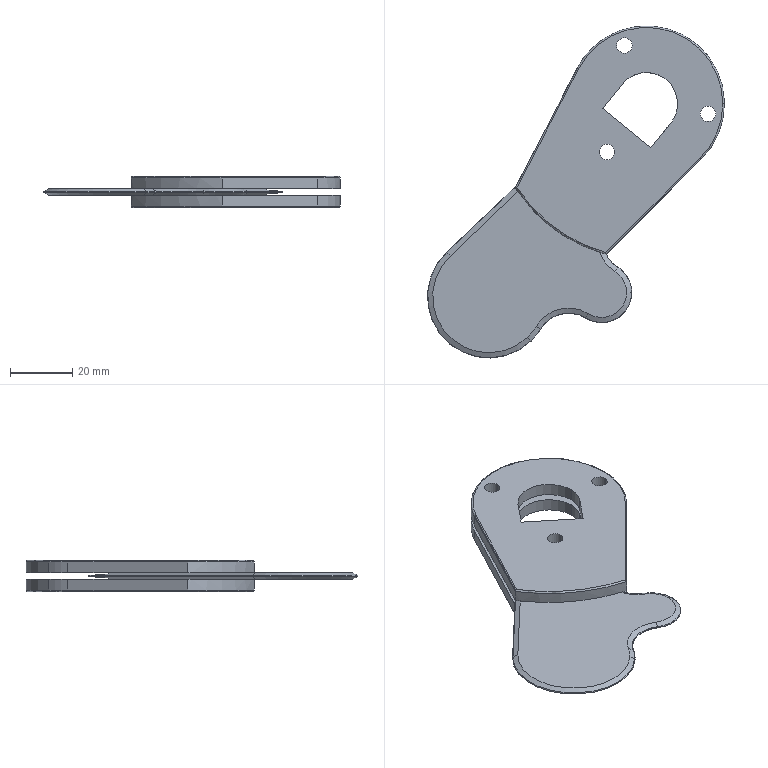Part | SolidWorks | features BaseBody 1 | 1 solid | 79 faces | box 95.327 x 106.627 x 10 mm | volume 27303 mm3 | cylinder 32 | plane 21 | torus 14 | cone 12 | commonest cylinder face diameters 5 x10 1 x8 0.5 x4 20 x4 50 x4 100 x2